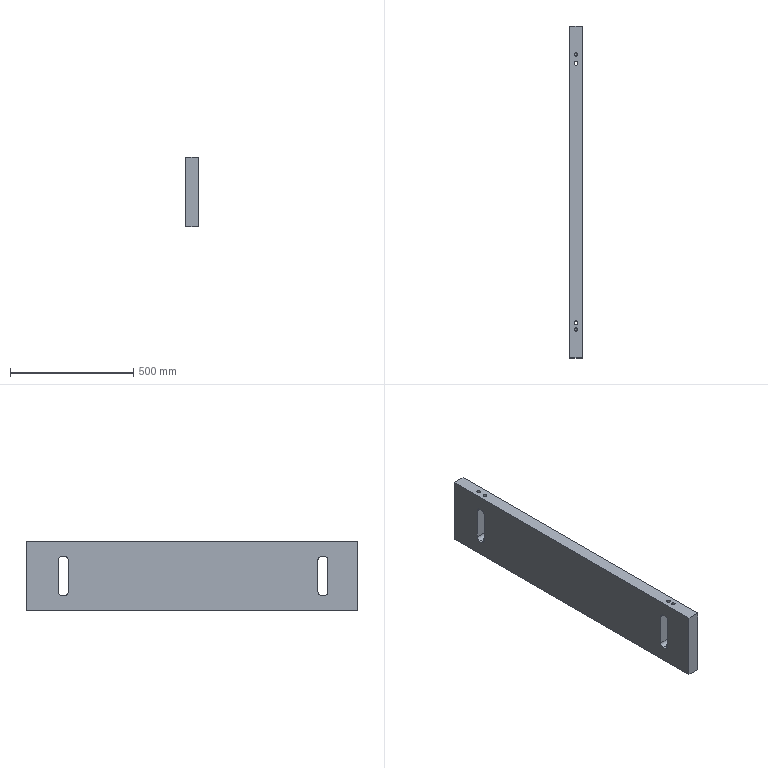Part | NX | features 29 2 | 1 solid | 38 faces | box 50 x 1345 x 280.5 mm | volume 18169896 mm3 | plane 18 | cylinder 16 | cone 4 | commonest cylinder face diameters 30 x8 14.1 x4 16.001 x4
STEP:
#1=CARTESIAN_POINT('',(3953.754,516.5,-273.));
#2=VERTEX_POINT('',#1);
#3=CARTESIAN_POINT('',(3966.246,516.5,-273.));
#4=VERTEX_POINT('',#3);
#5=CARTESIAN_POINT('',(3953.754,516.5,-273.));
#6=CARTESIAN_POINT('',(3955.263,514.616,-273.));
#7=CARTESIAN_POINT('',(3959.987,512.383,-273.606));
#8=CARTESIAN_POINT('',(3964.737,514.616,-273.));
#9=CARTESIAN_POINT('',(3966.246,516.5,-273.));
#10=B_SPLINE_CURVE_WITH_KNOTS('',3,(#5,#6,#7,#8,#9),.UNSPECIFIED.,.F.,.F.,(4,1,4),(0.,0.007135,0.01427),.UNSPECIFIED.);
#11=EDGE_CURVE('',#2,#4,#10,.T.);
#12=ORIENTED_EDGE('',*,*,#11,.F.);
#13=CARTESIAN_POINT('',(3953.754,526.5,-273.));
#14=VERTEX_POINT('',#13);
#15=CARTESIAN_POINT('',(3960.,521.5,-273.));
#16=DIRECTION('',(0.,0.,1.));
#17=DIRECTION('',(1.,0.,0.));
#18=AXIS2_PLACEMENT_3D('',#15,#16,#17);
#19=CIRCLE('',#18,8.001);
#20=EDGE_CURVE('',#14,#2,#19,.T.);
#21=ORIENTED_EDGE('',*,*,#20,.F.);
#22=CARTESIAN_POINT('',(3966.246,526.5,-273.));
#23=VERTEX_POINT('',#22);
#24=CARTESIAN_POINT('',(3966.246,526.5,-273.));
#25=CARTESIAN_POINT('',(3964.737,528.384,-273.));
#26=CARTESIAN_POINT('',(3960.013,530.617,-273.606));
#27=CARTESIAN_POINT('',(3955.263,528.384,-273.));
#28=CARTESIAN_POINT('',(3953.754,526.5,-273.));
#29=B_SPLINE_CURVE_WITH_KNOTS('',3,(#24,#25,#26,#27,#28),.UNSPECIFIED.,.F.,.F.,(4,1,4),(0.,0.007135,0.01427),.UNSPECIFIED.);
#30=EDGE_CURVE('',#23,#14,#29,.T.);
#31=ORIENTED_EDGE('',*,*,#30,.F.);
#32=CARTESIAN_POINT('',(3960.,521.5,-273.));
#33=DIRECTION('',(0.,0.,1.));
#34=DIRECTION('',(1.,0.,0.));
#35=AXIS2_PLACEMENT_3D('',#32,#33,#34);
#36=CIRCLE('',#35,8.001);
#37=EDGE_CURVE('',#4,#23,#36,.T.);
#38=ORIENTED_EDGE('',*,*,#37,.F.);
#39=EDGE_LOOP('',(#12,#21,#31,#38));
#40=FACE_BOUND('',#39,.T.);
#41=CARTESIAN_POINT('',(3968.001,521.5,-213.));
#42=VERTEX_POINT('',#41);
#43=CARTESIAN_POINT('',(3960.,521.5,-213.));
#44=DIRECTION('',(0.,0.,1.));
#45=DIRECTION('',(1.,0.,0.));
#46=AXIS2_PLACEMENT_3D('',#43,#44,#45);
#47=CIRCLE('',#46,8.001);
#48=EDGE_CURVE('',#42,#42,#47,.T.);
#49=ORIENTED_EDGE('',*,*,#48,.T.);
#50=EDGE_LOOP('',(#49));
#51=FACE_BOUND('',#50,.T.);
#52=CARTESIAN_POINT('',(3960.,521.5,-213.));
#53=DIRECTION('',(0.,0.,-1.));
#54=DIRECTION('',(-1.,0.,0.));
#55=AXIS2_PLACEMENT_3D('',#52,#53,#54);
#56=CYLINDRICAL_SURFACE('',#55,8.001);
#57=ADVANCED_FACE('',(#40,#51),#56,.F.);
#58=CARTESIAN_POINT('',(3960.,-557.5,-449.5));
#59=VERTEX_POINT('',#58);
#60=VERTEX_LOOP('',#59);
#61=FACE_BOUND('',#60,.T.);
#62=CARTESIAN_POINT('',(3967.05,-557.5,-456.55));
#63=VERTEX_POINT('',#62);
#64=CARTESIAN_POINT('',(3960.,-557.5,-456.55));
#65=DIRECTION('',(0.,0.,1.));
#66=DIRECTION('',(1.,0.,0.));
#67=AXIS2_PLACEMENT_3D('',#64,#65,#66);
#68=CIRCLE('',#67,7.05);
#69=EDGE_CURVE('',#63,#63,#68,.T.);
#70=ORIENTED_EDGE('',*,*,#69,.F.);
#71=EDGE_LOOP('',(#70));
#72=FACE_BOUND('',#71,.T.);
#73=CARTESIAN_POINT('',(3960.,-557.5,-456.55));
#74=DIRECTION('',(0.,0.,-1.));
#75=DIRECTION('',(1.,0.,0.));
#76=AXIS2_PLACEMENT_3D('',#73,#74,#75);
#77=CONICAL_SURFACE('',#76,7.05,0.7854);
#78=ADVANCED_FACE('',(#61,#72),#77,.F.);
#79=CARTESIAN_POINT('',(3960.,557.5,-449.5));
#80=VERTEX_POINT('',#79);
#81=VERTEX_LOOP('',#80);
#82=FACE_BOUND('',#81,.T.);
#83=CARTESIAN_POINT('',(3967.05,557.5,-456.55));
#84=VERTEX_POINT('',#83);
#85=CARTESIAN_POINT('',(3960.,557.5,-456.55));
#86=DIRECTION('',(0.,0.,1.));
#87=DIRECTION('',(1.,0.,0.));
#88=AXIS2_PLACEMENT_3D('',#85,#86,#87);
#89=CIRCLE('',#88,7.05);
#90=EDGE_CURVE('',#84,#84,#89,.T.);
#91=ORIENTED_EDGE('',*,*,#90,.F.);
#92=EDGE_LOOP('',(#91));
#93=FACE_BOUND('',#92,.T.);
#94=CARTESIAN_POINT('',(3960.,557.5,-456.55));
#95=DIRECTION('',(0.,0.,-1.));
#96=DIRECTION('',(1.,0.,0.));
#97=AXIS2_PLACEMENT_3D('',#94,#95,#96);
#98=CONICAL_SURFACE('',#97,7.05,0.7854);
#99=ADVANCED_FACE('',(#82,#93),#98,.F.);
#100=ORIENTED_EDGE('',*,*,#69,.T.);
#101=EDGE_LOOP('',(#100));
#102=FACE_BOUND('',#101,.T.);
#103=CARTESIAN_POINT('',(3967.05,-557.5,-493.5));
#104=VERTEX_POINT('',#103);
#105=CARTESIAN_POINT('',(3960.,-557.5,-493.5));
#106=DIRECTION('',(0.,0.,1.));
#107=DIRECTION('',(1.,0.,0.));
#108=AXIS2_PLACEMENT_3D('',#105,#106,#107);
#109=CIRCLE('',#108,7.05);
#110=EDGE_CURVE('',#104,#104,#109,.T.);
#111=ORIENTED_EDGE('',*,*,#110,.F.);
#112=EDGE_LOOP('',(#111));
#113=FACE_BOUND('',#112,.T.);
#114=CARTESIAN_POINT('',(3960.,-557.5,-493.5));
#115=DIRECTION('',(0.,0.,1.));
#116=DIRECTION('',(-1.,0.,0.));
#117=AXIS2_PLACEMENT_3D('',#114,#115,#116);
#118=CYLINDRICAL_SURFACE('',#117,7.05);
#119=ADVANCED_FACE('',(#102,#113),#118,.F.);
#120=ORIENTED_EDGE('',*,*,#90,.T.);
#121=EDGE_LOOP('',(#120));
#122=FACE_BOUND('',#121,.T.);
#123=CARTESIAN_POINT('',(3967.05,557.5,-493.5));
#124=VERTEX_POINT('',#123);
#125=CARTESIAN_POINT('',(3960.,557.5,-493.5));
#126=DIRECTION('',(0.,0.,1.));
#127=DIRECTION('',(1.,0.,0.));
#128=AXIS2_PLACEMENT_3D('',#125,#126,#127);
#129=CIRCLE('',#128,7.05);
#130=EDGE_CURVE('',#124,#124,#129,.T.);
#131=ORIENTED_EDGE('',*,*,#130,.F.);
#132=EDGE_LOOP('',(#131));
#133=FACE_BOUND('',#132,.T.);
#134=CARTESIAN_POINT('',(3960.,557.5,-493.5));
#135=DIRECTION('',(0.,0.,1.));
#136=DIRECTION('',(-1.,0.,0.));
#137=AXIS2_PLACEMENT_3D('',#134,#135,#136);
#138=CYLINDRICAL_SURFACE('',#137,7.05);
#139=ADVANCED_FACE('',(#122,#133),#138,.F.);
#140=CARTESIAN_POINT('',(3968.001,-530.5,-493.5));
#141=VERTEX_POINT('',#140);
#142=CARTESIAN_POINT('',(3960.,-530.5,-493.5));
#143=DIRECTION('',(0.,0.,1.));
#144=DIRECTION('',(1.,0.,0.));
#145=AXIS2_PLACEMENT_3D('',#142,#143,#144);
#146=CIRCLE('',#145,8.001);
#147=EDGE_CURVE('',#141,#141,#146,.T.);
#148=ORIENTED_EDGE('',*,*,#147,.F.);
#149=EDGE_LOOP('',(#148));
#150=FACE_BOUND('',#149,.T.);
#151=CARTESIAN_POINT('',(3953.754,-535.5,-433.));
#152=VERTEX_POINT('',#151);
#153=CARTESIAN_POINT('',(3953.754,-525.5,-433.));
#154=VERTEX_POINT('',#153);
#155=CARTESIAN_POINT('',(3960.,-530.5,-433.));
#156=DIRECTION('',(0.,0.,-1.));
#157=DIRECTION('',(-1.,0.,0.));
#158=AXIS2_PLACEMENT_3D('',#155,#156,#157);
#159=CIRCLE('',#158,8.001);
#160=EDGE_CURVE('',#152,#154,#159,.T.);
#161=ORIENTED_EDGE('',*,*,#160,.F.);
#162=CARTESIAN_POINT('',(3966.246,-535.5,-433.));
#163=VERTEX_POINT('',#162);
#164=CARTESIAN_POINT('',(3966.246,-535.5,-433.));
#165=CARTESIAN_POINT('',(3964.737,-537.384,-433.));
#166=CARTESIAN_POINT('',(3960.013,-539.617,-432.394));
#167=CARTESIAN_POINT('',(3955.263,-537.384,-433.));
#168=CARTESIAN_POINT('',(3953.754,-535.5,-433.));
#169=B_SPLINE_CURVE_WITH_KNOTS('',3,(#164,#165,#166,#167,#168),.UNSPECIFIED.,.F.,.F.,(4,1,4),(0.,0.007135,0.01427),.UNSPECIFIED.);
#170=EDGE_CURVE('',#163,#152,#169,.T.);
#171=ORIENTED_EDGE('',*,*,#170,.F.);
#172=CARTESIAN_POINT('',(3966.246,-525.5,-433.));
#173=VERTEX_POINT('',#172);
#174=CARTESIAN_POINT('',(3960.,-530.5,-433.));
#175=DIRECTION('',(0.,0.,-1.));
#176=DIRECTION('',(-1.,0.,0.));
#177=AXIS2_PLACEMENT_3D('',#174,#175,#176);
#178=CIRCLE('',#177,8.001);
#179=EDGE_CURVE('',#173,#163,#178,.T.);
#180=ORIENTED_EDGE('',*,*,#179,.F.);
#181=CARTESIAN_POINT('',(3953.754,-525.5,-433.));
#182=CARTESIAN_POINT('',(3955.263,-523.616,-433.));
#183=CARTESIAN_POINT('',(3959.987,-521.383,-432.394));
#184=CARTESIAN_POINT('',(3964.737,-523.616,-433.));
#185=CARTESIAN_POINT('',(3966.246,-525.5,-433.));
#186=B_SPLINE_CURVE_WITH_KNOTS('',3,(#181,#182,#183,#184,#185),.UNSPECIFIED.,.F.,.F.,(4,1,4),(0.,0.007135,0.01427),.UNSPECIFIED.);
#187=EDGE_CURVE('',#154,#173,#186,.T.);
#188=ORIENTED_EDGE('',*,*,#187,.F.);
#189=EDGE_LOOP('',(#161,#171,#180,#188));
#190=FACE_BOUND('',#189,.T.);
#191=CARTESIAN_POINT('',(3960.,-530.5,-493.5));
#192=DIRECTION('',(0.,0.,1.));
#193=DIRECTION('',(-1.,0.,0.));
#194=AXIS2_PLACEMENT_3D('',#191,#192,#193);
#195=CYLINDRICAL_SURFACE('',#194,8.001);
#196=ADVANCED_FACE('',(#150,#190),#195,.F.);
#197=CARTESIAN_POINT('',(3968.001,521.5,-493.5));
#198=VERTEX_POINT('',#197);
#199=CARTESIAN_POINT('',(3960.,521.5,-493.5));
#200=DIRECTION('',(0.,0.,1.));
#201=DIRECTION('',(1.,0.,0.));
#202=AXIS2_PLACEMENT_3D('',#199,#200,#201);
#203=CIRCLE('',#202,8.001);
#204=EDGE_CURVE('',#198,#198,#203,.T.);
#205=ORIENTED_EDGE('',*,*,#204,.F.);
#206=EDGE_LOOP('',(#205));
#207=FACE_BOUND('',#206,.T.);
#208=CARTESIAN_POINT('',(3953.754,516.5,-433.));
#209=VERTEX_POINT('',#208);
#210=CARTESIAN_POINT('',(3953.754,526.5,-433.));
#211=VERTEX_POINT('',#210);
#212=CARTESIAN_POINT('',(3960.,521.5,-433.));
#213=DIRECTION('',(0.,0.,-1.));
#214=DIRECTION('',(-1.,0.,0.));
#215=AXIS2_PLACEMENT_3D('',#212,#213,#214);
#216=CIRCLE('',#215,8.001);
#217=EDGE_CURVE('',#209,#211,#216,.T.);
#218=ORIENTED_EDGE('',*,*,#217,.F.);
#219=CARTESIAN_POINT('',(3966.246,516.5,-433.));
#220=VERTEX_POINT('',#219);
#221=CARTESIAN_POINT('',(3966.246,516.5,-433.));
#222=CARTESIAN_POINT('',(3964.737,514.616,-433.));
#223=CARTESIAN_POINT('',(3960.013,512.383,-432.394));
#224=CARTESIAN_POINT('',(3955.263,514.616,-433.));
#225=CARTESIAN_POINT('',(3953.754,516.5,-433.));
#226=B_SPLINE_CURVE_WITH_KNOTS('',3,(#221,#222,#223,#224,#225),.UNSPECIFIED.,.F.,.F.,(4,1,4),(0.,0.007135,0.01427),.UNSPECIFIED.);
#227=EDGE_CURVE('',#220,#209,#226,.T.);
#228=ORIENTED_EDGE('',*,*,#227,.F.);
#229=CARTESIAN_POINT('',(3966.246,526.5,-433.));
#230=VERTEX_POINT('',#229);
#231=CARTESIAN_POINT('',(3960.,521.5,-433.));
#232=DIRECTION('',(0.,0.,-1.));
#233=DIRECTION('',(-1.,0.,0.));
#234=AXIS2_PLACEMENT_3D('',#231,#232,#233);
#235=CIRCLE('',#234,8.001);
#236=EDGE_CURVE('',#230,#220,#235,.T.);
#237=ORIENTED_EDGE('',*,*,#236,.F.);
#238=CARTESIAN_POINT('',(3953.754,526.5,-433.));
#239=CARTESIAN_POINT('',(3955.263,528.384,-433.));
#240=CARTESIAN_POINT('',(3959.987,530.617,-432.394));
#241=CARTESIAN_POINT('',(3964.737,528.384,-433.));
#242=CARTESIAN_POINT('',(3966.246,526.5,-433.));
#243=B_SPLINE_CURVE_WITH_KNOTS('',3,(#238,#239,#240,#241,#242),.UNSPECIFIED.,.F.,.F.,(4,1,4),(0.,0.007135,0.01427),.UNSPECIFIED.);
#244=EDGE_CURVE('',#211,#230,#243,.T.);
#245=ORIENTED_EDGE('',*,*,#244,.F.);
#246=EDGE_LOOP('',(#218,#228,#237,#245));
#247=FACE_BOUND('',#246,.T.);
#248=CARTESIAN_POINT('',(3960.,521.5,-493.5));
#249=DIRECTION('',(0.,0.,1.));
#250=DIRECTION('',(-1.,0.,0.));
#251=AXIS2_PLACEMENT_3D('',#248,#249,#250);
#252=CYLINDRICAL_SURFACE('',#251,8.001);
#253=ADVANCED_FACE('',(#207,#247),#252,.F.);
#254=CARTESIAN_POINT('',(3960.,-557.5,-257.));
#255=VERTEX_POINT('',#254);
#256=VERTEX_LOOP('',#255);
#257=FACE_BOUND('',#256,.T.);
#258=CARTESIAN_POINT('',(3952.95,-557.5,-249.95));
#259=VERTEX_POINT('',#258);
#260=CARTESIAN_POINT('',(3960.,-557.5,-249.95));
#261=DIRECTION('',(0.,0.,-1.));
#262=DIRECTION('',(-1.,0.,0.));
#263=AXIS2_PLACEMENT_3D('',#260,#261,#262);
#264=CIRCLE('',#263,7.05);
#265=EDGE_CURVE('',#259,#259,#264,.T.);
#266=ORIENTED_EDGE('',*,*,#265,.F.);
#267=EDGE_LOOP('',(#266));
#268=FACE_BOUND('',#267,.T.);
#269=CARTESIAN_POINT('',(3960.,-557.5,-249.95));
#270=DIRECTION('',(0.,0.,1.));
#271=DIRECTION('',(-1.,0.,0.));
#272=AXIS2_PLACEMENT_3D('',#269,#270,#271);
#273=CONICAL_SURFACE('',#272,7.05,0.7854);
#274=ADVANCED_FACE('',(#257,#268),#273,.F.);
#275=CARTESIAN_POINT('',(3960.,557.5,-257.));
#276=VERTEX_POINT('',#275);
#277=VERTEX_LOOP('',#276);
#278=FACE_BOUND('',#277,.T.);
#279=CARTESIAN_POINT('',(3952.95,557.5,-249.95));
#280=VERTEX_POINT('',#279);
#281=CARTESIAN_POINT('',(3960.,557.5,-249.95));
#282=DIRECTION('',(0.,0.,-1.));
#283=DIRECTION('',(-1.,0.,0.));
#284=AXIS2_PLACEMENT_3D('',#281,#282,#283);
#285=CIRCLE('',#284,7.05);
#286=EDGE_CURVE('',#280,#280,#285,.T.);
#287=ORIENTED_EDGE('',*,*,#286,.F.);
#288=EDGE_LOOP('',(#287));
#289=FACE_BOUND('',#288,.T.);
#290=CARTESIAN_POINT('',(3960.,557.5,-249.95));
#291=DIRECTION('',(0.,0.,1.));
#292=DIRECTION('',(-1.,0.,0.));
#293=AXIS2_PLACEMENT_3D('',#290,#291,#292);
#294=CONICAL_SURFACE('',#293,7.05,0.7854);
#295=ADVANCED_FACE('',(#278,#289),#294,.F.);
#296=CARTESIAN_POINT('',(3985.,-525.5,-433.));
#297=VERTEX_POINT('',#296);
#298=CARTESIAN_POINT('',(3960.,-525.5,-433.));
#299=DIRECTION('',(1.,0.,0.));
#300=VECTOR('',#299,1000.);
#301=LINE('',#298,#300);
#302=EDGE_CURVE('',#173,#297,#301,.T.);
#303=ORIENTED_EDGE('',*,*,#302,.F.);
#304=ORIENTED_EDGE('',*,*,#179,.T.);
#305=CARTESIAN_POINT('',(3985.,-535.5,-433.));
#306=VERTEX_POINT('',#305);
#307=CARTESIAN_POINT('',(3960.,-535.5,-433.));
#308=DIRECTION('',(-1.,0.,0.));
#309=VECTOR('',#308,1000.);
#310=LINE('',#307,#309);
#311=EDGE_CURVE('',#306,#163,#310,.T.);
#312=ORIENTED_EDGE('',*,*,#311,.F.);
#313=CARTESIAN_POINT('',(3985.,193.,-433.));
#314=DIRECTION('',(0.,1.,0.));
#315=VECTOR('',#314,1000.);
#316=LINE('',#313,#315);
#317=EDGE_CURVE('',#306,#297,#316,.T.);
#318=ORIENTED_EDGE('',*,*,#317,.T.);
#319=EDGE_LOOP('',(#303,#304,#312,#318));
#320=FACE_BOUND('',#319,.T.);
#321=CARTESIAN_POINT('',(3960.,-521.5,-433.));
#322=DIRECTION('',(0.,0.,-1.));
#323=DIRECTION('',(-1.,0.,0.));
#324=AXIS2_PLACEMENT_3D('',#321,#322,#323);
#325=PLANE('',#324);
#326=ADVANCED_FACE('',(#320),#325,.F.);
#327=CARTESIAN_POINT('',(3985.,526.5,-433.));
#328=VERTEX_POINT('',#327);
#329=CARTESIAN_POINT('',(3960.,526.5,-433.));
#330=DIRECTION('',(-1.,0.,0.));
#331=VECTOR('',#330,1000.);
#332=LINE('',#329,#331);
#333=EDGE_CURVE('',#328,#230,#332,.T.);
#334=ORIENTED_EDGE('',*,*,#333,.T.);
#335=ORIENTED_EDGE('',*,*,#236,.T.);
#336=CARTESIAN_POINT('',(3985.,516.5,-433.));
#337=VERTEX_POINT('',#336);
#338=CARTESIAN_POINT('',(3960.,516.5,-433.));
#339=DIRECTION('',(1.,0.,0.));
#340=VECTOR('',#339,1000.);
#341=LINE('',#338,#340);
#342=EDGE_CURVE('',#220,#337,#341,.T.);
#343=ORIENTED_EDGE('',*,*,#342,.T.);
#344=CARTESIAN_POINT('',(3985.,193.,-433.));
#345=DIRECTION('',(0.,1.,0.));
#346=VECTOR('',#345,1000.);
#347=LINE('',#344,#346);
#348=EDGE_CURVE('',#337,#328,#347,.T.);
#349=ORIENTED_EDGE('',*,*,#348,.T.);
#350=EDGE_LOOP('',(#334,#335,#343,#349));
#351=FACE_BOUND('',#350,.T.);
#352=CARTESIAN_POINT('',(3960.,521.5,-433.));
#353=DIRECTION('',(0.,0.,-1.));
#354=DIRECTION('',(-1.,0.,0.));
#355=AXIS2_PLACEMENT_3D('',#352,#353,#354);
#356=PLANE('',#355);
#357=ADVANCED_FACE('',(#351),#356,.F.);
#358=ORIENTED_EDGE('',*,*,#147,.T.);
#359=EDGE_LOOP('',(#358));
#360=FACE_BOUND('',#359,.T.);
#361=ORIENTED_EDGE('',*,*,#130,.T.);
#362=EDGE_LOOP('',(#361));
#363=FACE_BOUND('',#362,.T.);
#364=CARTESIAN_POINT('',(3935.,672.5,-493.5));
#365=VERTEX_POINT('',#364);
#366=CARTESIAN_POINT('',(3935.,-672.5,-493.5));
#367=VERTEX_POINT('',#366);
#368=CARTESIAN_POINT('',(3935.,193.,-493.5));
#369=DIRECTION('',(0.,-1.,0.));
#370=VECTOR('',#369,1000.);
#371=LINE('',#368,#370);
#372=EDGE_CURVE('',#365,#367,#371,.T.);
#373=ORIENTED_EDGE('',*,*,#372,.F.);
#374=CARTESIAN_POINT('',(3985.,672.5,-493.5));
#375=VERTEX_POINT('',#374);
#376=CARTESIAN_POINT('',(1822.5,672.5,-493.5));
#377=DIRECTION('',(1.,0.,0.));
#378=VECTOR('',#377,1000.);
#379=LINE('',#376,#378);
#380=EDGE_CURVE('',#365,#375,#379,.T.);
#381=ORIENTED_EDGE('',*,*,#380,.T.);
#382=CARTESIAN_POINT('',(3985.,-672.5,-493.5));
#383=VERTEX_POINT('',#382);
#384=CARTESIAN_POINT('',(3985.,193.,-493.5));
#385=DIRECTION('',(0.,1.,0.));
#386=VECTOR('',#385,1000.);
#387=LINE('',#384,#386);
#388=EDGE_CURVE('',#383,#375,#387,.T.);
#389=ORIENTED_EDGE('',*,*,#388,.F.);
#390=CARTESIAN_POINT('',(4325.,-672.5,-493.5));
#391=DIRECTION('',(-1.,0.,0.));
#392=VECTOR('',#391,1000.);
#393=LINE('',#390,#392);
#394=EDGE_CURVE('',#383,#367,#393,.T.);
#395=ORIENTED_EDGE('',*,*,#394,.T.);
#396=EDGE_LOOP('',(#373,#381,#389,#395));
#397=FACE_BOUND('',#396,.T.);
#398=ORIENTED_EDGE('',*,*,#110,.T.);
#399=EDGE_LOOP('',(#398));
#400=FACE_BOUND('',#399,.T.);
#401=ORIENTED_EDGE('',*,*,#204,.T.);
#402=EDGE_LOOP('',(#401));
#403=FACE_BOUND('',#402,.T.);
#404=CARTESIAN_POINT('',(1945.,0.,-493.5));
#405=DIRECTION('',(0.,0.,-1.));
#406=DIRECTION('',(1.,0.,0.));
#407=AXIS2_PLACEMENT_3D('',#404,#405,#406);
#408=PLANE('',#407);
#409=ADVANCED_FACE('',(#360,#363,#397,#400,#403),#408,.T.);
#410=CARTESIAN_POINT('',(3935.,-525.5,-433.));
#411=VERTEX_POINT('',#410);
#412=CARTESIAN_POINT('',(3960.,-525.5,-433.));
#413=DIRECTION('',(1.,0.,0.));
#414=VECTOR('',#413,1000.);
#415=LINE('',#412,#414);
#416=EDGE_CURVE('',#411,#154,#415,.T.);
#417=ORIENTED_EDGE('',*,*,#416,.T.);
#418=ORIENTED_EDGE('',*,*,#187,.T.);
#419=ORIENTED_EDGE('',*,*,#302,.T.);
#420=CARTESIAN_POINT('',(3985.,-510.5,-418.));
#421=VERTEX_POINT('',#420);
#422=CARTESIAN_POINT('',(3985.,-525.5,-418.));
#423=DIRECTION('',(1.,0.,0.));
#424=DIRECTION('',(0.,0.,-1.));
#425=AXIS2_PLACEMENT_3D('',#422,#423,#424);
#426=CIRCLE('',#425,15.);
#427=EDGE_CURVE('',#297,#421,#426,.T.);
#428=ORIENTED_EDGE('',*,*,#427,.T.);
#429=CARTESIAN_POINT('',(3935.,-510.5,-418.));
#430=VERTEX_POINT('',#429);
#431=CARTESIAN_POINT('',(3960.,-510.5,-418.));
#432=DIRECTION('',(-1.,0.,0.));
#433=VECTOR('',#432,1000.);
#434=LINE('',#431,#433);
#435=EDGE_CURVE('',#421,#430,#434,.T.);
#436=ORIENTED_EDGE('',*,*,#435,.T.);
#437=CARTESIAN_POINT('',(3935.,-525.5,-418.));
#438=DIRECTION('',(-1.,0.,0.));
#439=DIRECTION('',(0.,0.,1.));
#440=AXIS2_PLACEMENT_3D('',#437,#438,#439);
#441=CIRCLE('',#440,15.);
#442=EDGE_CURVE('',#430,#411,#441,.T.);
#443=ORIENTED_EDGE('',*,*,#442,.T.);
#444=EDGE_LOOP('',(#417,#418,#419,#428,#436,#443));
#445=FACE_BOUND('',#444,.T.);
#446=CARTESIAN_POINT('',(3960.,-525.5,-418.));
#447=DIRECTION('',(1.,0.,0.));
#448=DIRECTION('',(0.,0.,-1.));
#449=AXIS2_PLACEMENT_3D('',#446,#447,#448);
#450=CYLINDRICAL_SURFACE('',#449,15.);
#451=ADVANCED_FACE('',(#445),#450,.F.);
#452=CARTESIAN_POINT('',(3935.,-535.5,-433.));
#453=VERTEX_POINT('',#452);
#454=CARTESIAN_POINT('',(3960.,-535.5,-433.));
#455=DIRECTION('',(-1.,0.,0.));
#456=VECTOR('',#455,1000.);
#457=LINE('',#454,#456);
#458=EDGE_CURVE('',#152,#453,#457,.T.);
#459=ORIENTED_EDGE('',*,*,#458,.F.);
#460=ORIENTED_EDGE('',*,*,#160,.T.);
#461=ORIENTED_EDGE('',*,*,#416,.F.);
#462=CARTESIAN_POINT('',(3935.,193.,-433.));
#463=DIRECTION('',(0.,-1.,0.));
#464=VECTOR('',#463,1000.);
#465=LINE('',#462,#464);
#466=EDGE_CURVE('',#411,#453,#465,.T.);
#467=ORIENTED_EDGE('',*,*,#466,.T.);
#468=EDGE_LOOP('',(#459,#460,#461,#467));
#469=FACE_BOUND('',#468,.T.);
#470=CARTESIAN_POINT('',(3960.,-521.5,-433.));
#471=DIRECTION('',(0.,0.,-1.));
#472=DIRECTION('',(-1.,0.,0.));
#473=AXIS2_PLACEMENT_3D('',#470,#471,#472);
#474=PLANE('',#473);
#475=ADVANCED_FACE('',(#469),#474,.F.);
#476=ORIENTED_EDGE('',*,*,#311,.T.);
#477=ORIENTED_EDGE('',*,*,#170,.T.);
#478=ORIENTED_EDGE('',*,*,#458,.T.);
#479=CARTESIAN_POINT('',(3935.,-550.5,-418.));
#480=VERTEX_POINT('',#479);
#481=CARTESIAN_POINT('',(3935.,-535.5,-418.));
#482=DIRECTION('',(-1.,0.,0.));
#483=DIRECTION('',(0.,0.,1.));
#484=AXIS2_PLACEMENT_3D('',#481,#482,#483);
#485=CIRCLE('',#484,15.);
#486=EDGE_CURVE('',#453,#480,#485,.T.);
#487=ORIENTED_EDGE('',*,*,#486,.T.);
#488=CARTESIAN_POINT('',(3985.,-550.5,-418.));
#489=VERTEX_POINT('',#488);
#490=CARTESIAN_POINT('',(3960.,-550.5,-418.));
#491=DIRECTION('',(1.,0.,0.));
#492=VECTOR('',#491,1000.);
#493=LINE('',#490,#492);
#494=EDGE_CURVE('',#480,#489,#493,.T.);
#495=ORIENTED_EDGE('',*,*,#494,.T.);
#496=CARTESIAN_POINT('',(3985.,-535.5,-418.));
#497=DIRECTION('',(1.,0.,0.));
#498=DIRECTION('',(0.,0.,-1.));
#499=AXIS2_PLACEMENT_3D('',#496,#497,#498);
#500=CIRCLE('',#499,15.);
#501=EDGE_CURVE('',#489,#306,#500,.T.);
#502=ORIENTED_EDGE('',*,*,#501,.T.);
#503=EDGE_LOOP('',(#476,#477,#478,#487,#495,#502));
#504=FACE_BOUND('',#503,.T.);
#505=CARTESIAN_POINT('',(3960.,-535.5,-418.));
#506=DIRECTION('',(-1.,0.,0.));
#507=DIRECTION('',(0.,0.,1.));
#508=AXIS2_PLACEMENT_3D('',#505,#506,#507);
#509=CYLINDRICAL_SURFACE('',#508,15.);
#510=ADVANCED_FACE('',(#504),#509,.F.);
#511=CARTESIAN_POINT('',(3935.,526.5,-433.));
#512=VERTEX_POINT('',#511);
#513=CARTESIAN_POINT('',(3960.,526.5,-433.));
#514=DIRECTION('',(-1.,0.,0.));
#515=VECTOR('',#514,1000.);
#516=LINE('',#513,#515);
#517=EDGE_CURVE('',#211,#512,#516,.T.);
#518=ORIENTED_EDGE('',*,*,#517,.F.);
#519=ORIENTED_EDGE('',*,*,#244,.T.);
#520=ORIENTED_EDGE('',*,*,#333,.F.);
#521=CARTESIAN_POINT('',(3985.,541.5,-418.));
#522=VERTEX_POINT('',#521);
#523=CARTESIAN_POINT('',(3985.,526.5,-418.));
#524=DIRECTION('',(1.,0.,0.));
#525=DIRECTION('',(0.,0.,-1.));
#526=AXIS2_PLACEMENT_3D('',#523,#524,#525);
#527=CIRCLE('',#526,15.);
#528=EDGE_CURVE('',#328,#522,#527,.T.);
#529=ORIENTED_EDGE('',*,*,#528,.T.);
#530=CARTESIAN_POINT('',(3935.,541.5,-418.));
#531=VERTEX_POINT('',#530);
#532=CARTESIAN_POINT('',(3960.,541.5,-418.));
#533=DIRECTION('',(1.,0.,0.));
#534=VECTOR('',#533,1000.);
#535=LINE('',#532,#534);
#536=EDGE_CURVE('',#531,#522,#535,.T.);
#537=ORIENTED_EDGE('',*,*,#536,.F.);
#538=CARTESIAN_POINT('',(3935.,526.5,-418.));
#539=DIRECTION('',(-1.,0.,0.));
#540=DIRECTION('',(0.,0.,1.));
#541=AXIS2_PLACEMENT_3D('',#538,#539,#540);
#542=CIRCLE('',#541,15.);
#543=EDGE_CURVE('',#531,#512,#542,.T.);
#544=ORIENTED_EDGE('',*,*,#543,.T.);
#545=EDGE_LOOP('',(#518,#519,#520,#529,#537,#544));
#546=FACE_BOUND('',#545,.T.);
#547=CARTESIAN_POINT('',(3960.,526.5,-418.));
#548=DIRECTION('',(-1.,0.,0.));
#549=DIRECTION('',(0.,0.,1.));
#550=AXIS2_PLACEMENT_3D('',#547,#548,#549);
#551=CYLINDRICAL_SURFACE('',#550,15.);
#552=ADVANCED_FACE('',(#546),#551,.F.);
#553=CARTESIAN_POINT('',(3935.,516.5,-433.));
#554=VERTEX_POINT('',#553);
#555=CARTESIAN_POINT('',(3960.,516.5,-433.));
#556=DIRECTION('',(1.,0.,0.));
#557=VECTOR('',#556,1000.);
#558=LINE('',#555,#557);
#559=EDGE_CURVE('',#554,#209,#558,.T.);
#560=ORIENTED_EDGE('',*,*,#559,.T.);
#561=ORIENTED_EDGE('',*,*,#217,.T.);
#562=ORIENTED_EDGE('',*,*,#517,.T.);
#563=CARTESIAN_POINT('',(3935.,193.,-433.));
#564=DIRECTION('',(0.,-1.,0.));
#565=VECTOR('',#564,1000.);
#566=LINE('',#563,#565);
#567=EDGE_CURVE('',#512,#554,#566,.T.);
#568=ORIENTED_EDGE('',*,*,#567,.T.);
#569=EDGE_LOOP('',(#560,#561,#562,#568));
#570=FACE_BOUND('',#569,.T.);
#571=CARTESIAN_POINT('',(3960.,521.5,-433.));
#572=DIRECTION('',(0.,0.,-1.));
#573=DIRECTION('',(-1.,0.,0.));
#574=AXIS2_PLACEMENT_3D('',#571,#572,#573);
#575=PLANE('',#574);
#576=ADVANCED_FACE('',(#570),#575,.F.);
#577=ORIENTED_EDGE('',*,*,#342,.F.);
#578=ORIENTED_EDGE('',*,*,#227,.T.);
#579=ORIENTED_EDGE('',*,*,#559,.F.);
#580=CARTESIAN_POINT('',(3935.,501.5,-418.));
#581=VERTEX_POINT('',#580);
#582=CARTESIAN_POINT('',(3935.,516.5,-418.));
#583=DIRECTION('',(-1.,0.,0.));
#584=DIRECTION('',(0.,0.,1.));
#585=AXIS2_PLACEMENT_3D('',#582,#583,#584);
#586=CIRCLE('',#585,15.);
#587=EDGE_CURVE('',#554,#581,#586,.T.);
#588=ORIENTED_EDGE('',*,*,#587,.T.);
#589=CARTESIAN_POINT('',(3985.,501.5,-418.));
#590=VERTEX_POINT('',#589);
#591=CARTESIAN_POINT('',(3960.,501.5,-418.));
#592=DIRECTION('',(-1.,0.,0.));
#593=VECTOR('',#592,1000.);
#594=LINE('',#591,#593);
#595=EDGE_CURVE('',#590,#581,#594,.T.);
#596=ORIENTED_EDGE('',*,*,#595,.F.);
#597=CARTESIAN_POINT('',(3985.,516.5,-418.));
#598=DIRECTION('',(1.,0.,0.));
#599=DIRECTION('',(0.,0.,-1.));
#600=AXIS2_PLACEMENT_3D('',#597,#598,#599);
#601=CIRCLE('',#600,15.);
#602=EDGE_CURVE('',#590,#337,#601,.T.);
#603=ORIENTED_EDGE('',*,*,#602,.T.);
#604=EDGE_LOOP('',(#577,#578,#579,#588,#596,#603));
#605=FACE_BOUND('',#604,.T.);
#606=CARTESIAN_POINT('',(3960.,516.5,-418.));
#607=DIRECTION('',(1.,0.,0.));
#608=DIRECTION('',(0.,0.,-1.));
#609=AXIS2_PLACEMENT_3D('',#606,#607,#608);
#610=CYLINDRICAL_SURFACE('',#609,15.);
#611=ADVANCED_FACE('',(#605),#610,.F.);
#612=ORIENTED_EDGE('',*,*,#265,.T.);
#613=EDGE_LOOP('',(#612));
#614=FACE_BOUND('',#613,.T.);
#615=CARTESIAN_POINT('',(3967.05,-557.5,-213.));
#616=VERTEX_POINT('',#615);
#617=CARTESIAN_POINT('',(3960.,-557.5,-213.));
#618=DIRECTION('',(0.,0.,-1.));
#619=DIRECTION('',(1.,0.,0.));
#620=AXIS2_PLACEMENT_3D('',#617,#618,#619);
#621=CIRCLE('',#620,7.05);
#622=EDGE_CURVE('',#616,#616,#621,.T.);
#623=ORIENTED_EDGE('',*,*,#622,.F.);
#624=EDGE_LOOP('',(#623));
#625=FACE_BOUND('',#624,.T.);
#626=CARTESIAN_POINT('',(3960.,-557.5,-213.));
#627=DIRECTION('',(0.,0.,-1.));
#628=DIRECTION('',(-1.,0.,0.));
#629=AXIS2_PLACEMENT_3D('',#626,#627,#628);
#630=CYLINDRICAL_SURFACE('',#629,7.05);
#631=ADVANCED_FACE('',(#614,#625),#630,.F.);
#632=ORIENTED_EDGE('',*,*,#380,.F.);
#633=CARTESIAN_POINT('',(3935.,672.5,-213.));
#634=VERTEX_POINT('',#633);
#635=CARTESIAN_POINT('',(3935.,672.5,-205.5));
#636=DIRECTION('',(0.,0.,1.));
#637=VECTOR('',#636,1000.);
#638=LINE('',#635,#637);
#639=EDGE_CURVE('',#365,#634,#638,.T.);
#640=ORIENTED_EDGE('',*,*,#639,.T.);
#641=CARTESIAN_POINT('',(3985.,672.5,-213.));
#642=VERTEX_POINT('',#641);
#643=CARTESIAN_POINT('',(1822.5,672.5,-213.));
#644=DIRECTION('',(-1.,0.,0.));
#645=VECTOR('',#644,1000.);
#646=LINE('',#643,#645);
#647=EDGE_CURVE('',#642,#634,#646,.T.);
#648=ORIENTED_EDGE('',*,*,#647,.F.);
#649=CARTESIAN_POINT('',(3985.,672.5,-205.5));
#650=DIRECTION('',(0.,0.,1.));
#651=VECTOR('',#650,1000.);
#652=LINE('',#649,#651);
#653=EDGE_CURVE('',#375,#642,#652,.T.);
#654=ORIENTED_EDGE('',*,*,#653,.F.);
#655=EDGE_LOOP('',(#632,#640,#648,#654));
#656=FACE_BOUND('',#655,.T.);
#657=CARTESIAN_POINT('',(1822.5,672.5,91.));
#658=DIRECTION('',(0.,-1.,0.));
#659=DIRECTION('',(-1.,0.,0.));
#660=AXIS2_PLACEMENT_3D('',#657,#658,#659);
#661=PLANE('',#660);
#662=ADVANCED_FACE('',(#656),#661,.F.);
#663=ORIENTED_EDGE('',*,*,#394,.F.);
#664=CARTESIAN_POINT('',(3985.,-672.5,-213.));
#665=VERTEX_POINT('',#664);
#666=CARTESIAN_POINT('',(3985.,-672.5,-543.5));
#667=DIRECTION('',(0.,0.,1.));
#668=VECTOR('',#667,1000.);
#669=LINE('',#666,#668);
#670=EDGE_CURVE('',#383,#665,#669,.T.);
#671=ORIENTED_EDGE('',*,*,#670,.T.);
#672=CARTESIAN_POINT('',(3935.,-672.5,-213.));
#673=VERTEX_POINT('',#672);
#674=CARTESIAN_POINT('',(4325.,-672.5,-213.));
#675=DIRECTION('',(1.,0.,0.));
#676=VECTOR('',#675,1000.);
#677=LINE('',#674,#676);
#678=EDGE_CURVE('',#673,#665,#677,.T.);
#679=ORIENTED_EDGE('',*,*,#678,.F.);
#680=CARTESIAN_POINT('',(3935.,-672.5,-113.));
#681=DIRECTION('',(0.,0.,1.));
#682=VECTOR('',#681,1000.);
#683=LINE('',#680,#682);
#684=EDGE_CURVE('',#367,#673,#683,.T.);
#685=ORIENTED_EDGE('',*,*,#684,.F.);
#686=EDGE_LOOP('',(#663,#671,#679,#685));
#687=FACE_BOUND('',#686,.T.);
#688=CARTESIAN_POINT('',(4325.,-672.5,-113.));
#689=DIRECTION('',(0.,1.,0.));
#690=DIRECTION('',(1.,0.,0.));
#691=AXIS2_PLACEMENT_3D('',#688,#689,#690);
#692=PLANE('',#691);
#693=ADVANCED_FACE('',(#687),#692,.F.);
#694=CARTESIAN_POINT('',(3935.,-510.5,-288.));
#695=VERTEX_POINT('',#694);
#696=CARTESIAN_POINT('',(3935.,-510.5,-205.5));
#697=DIRECTION('',(0.,0.,-1.));
#698=VECTOR('',#697,1000.);
#699=LINE('',#696,#698);
#700=EDGE_CURVE('',#695,#430,#699,.T.);
#701=ORIENTED_EDGE('',*,*,#700,.T.);
#702=ORIENTED_EDGE('',*,*,#435,.F.);
#703=CARTESIAN_POINT('',(3985.,-510.5,-288.));
#704=VERTEX_POINT('',#703);
#705=CARTESIAN_POINT('',(3985.,-510.5,-205.5));
#706=DIRECTION('',(0.,0.,1.));
#707=VECTOR('',#706,1000.);
#708=LINE('',#705,#707);
#709=EDGE_CURVE('',#421,#704,#708,.T.);
#710=ORIENTED_EDGE('',*,*,#709,.T.);
#711=CARTESIAN_POINT('',(3960.,-510.5,-288.));
#712=DIRECTION('',(1.,0.,0.));
#713=VECTOR('',#712,1000.);
#714=LINE('',#711,#713);
#715=EDGE_CURVE('',#695,#704,#714,.T.);
#716=ORIENTED_EDGE('',*,*,#715,.F.);
#717=EDGE_LOOP('',(#701,#702,#710,#716));
#718=FACE_BOUND('',#717,.T.);
#719=CARTESIAN_POINT('',(3960.,-510.5,-353.));
#720=DIRECTION('',(0.,1.,0.));
#721=DIRECTION('',(0.,0.,-1.));
#722=AXIS2_PLACEMENT_3D('',#719,#720,#721);
#723=PLANE('',#722);
#724=ADVANCED_FACE('',(#718),#723,.F.);
#725=CARTESIAN_POINT('',(3935.,-550.5,-288.));
#726=VERTEX_POINT('',#725);
#727=CARTESIAN_POINT('',(3935.,-550.5,-205.5));
#728=DIRECTION('',(0.,0.,1.));
#729=VECTOR('',#728,1000.);
#730=LINE('',#727,#729);
#731=EDGE_CURVE('',#480,#726,#730,.T.);
#732=ORIENTED_EDGE('',*,*,#731,.T.);
#733=CARTESIAN_POINT('',(3985.,-550.5,-288.));
#734=VERTEX_POINT('',#733);
#735=CARTESIAN_POINT('',(3960.,-550.5,-288.));
#736=DIRECTION('',(-1.,0.,0.));
#737=VECTOR('',#736,1000.);
#738=LINE('',#735,#737);
#739=EDGE_CURVE('',#734,#726,#738,.T.);
#740=ORIENTED_EDGE('',*,*,#739,.F.);
#741=CARTESIAN_POINT('',(3985.,-550.5,-205.5));
#742=DIRECTION('',(0.,0.,-1.));
#743=VECTOR('',#742,1000.);
#744=LINE('',#741,#743);
#745=EDGE_CURVE('',#734,#489,#744,.T.);
#746=ORIENTED_EDGE('',*,*,#745,.T.);
#747=ORIENTED_EDGE('',*,*,#494,.F.);
#748=EDGE_LOOP('',(#732,#740,#746,#747));
#749=FACE_BOUND('',#748,.T.);
#750=CARTESIAN_POINT('',(3960.,-550.5,-353.));
#751=DIRECTION('',(0.,-1.,0.));
#752=DIRECTION('',(0.,0.,1.));
#753=AXIS2_PLACEMENT_3D('',#750,#751,#752);
#754=PLANE('',#753);
#755=ADVANCED_FACE('',(#749),#754,.F.);
#756=CARTESIAN_POINT('',(3935.,501.5,-288.));
#757=VERTEX_POINT('',#756);
#758=CARTESIAN_POINT('',(3935.,501.5,-205.5));
#759=DIRECTION('',(0.,0.,1.));
#760=VECTOR('',#759,1000.);
#761=LINE('',#758,#760);
#762=EDGE_CURVE('',#581,#757,#761,.T.);
#763=ORIENTED_EDGE('',*,*,#762,.T.);
#764=CARTESIAN_POINT('',(3985.,501.5,-288.));
#765=VERTEX_POINT('',#764);
#766=CARTESIAN_POINT('',(3960.,501.5,-288.));
#767=DIRECTION('',(1.,0.,0.));
#768=VECTOR('',#767,1000.);
#769=LINE('',#766,#768);
#770=EDGE_CURVE('',#757,#765,#769,.T.);
#771=ORIENTED_EDGE('',*,*,#770,.T.);
#772=CARTESIAN_POINT('',(3985.,501.5,-205.5));
#773=DIRECTION('',(0.,0.,-1.));
#774=VECTOR('',#773,1000.);
#775=LINE('',#772,#774);
#776=EDGE_CURVE('',#765,#590,#775,.T.);
#777=ORIENTED_EDGE('',*,*,#776,.T.);
#778=ORIENTED_EDGE('',*,*,#595,.T.);
#779=EDGE_LOOP('',(#763,#771,#777,#778));
#780=FACE_BOUND('',#779,.T.);
#781=CARTESIAN_POINT('',(3960.,501.5,-353.));
#782=DIRECTION('',(0.,-1.,0.));
#783=DIRECTION('',(0.,0.,-1.));
#784=AXIS2_PLACEMENT_3D('',#781,#782,#783);
#785=PLANE('',#784);
#786=ADVANCED_FACE('',(#780),#785,.F.);
#787=CARTESIAN_POINT('',(3985.,516.5,-273.));
#788=VERTEX_POINT('',#787);
#789=CARTESIAN_POINT('',(3985.,516.5,-288.));
#790=DIRECTION('',(1.,0.,0.));
#791=DIRECTION('',(0.,0.,-1.));
#792=AXIS2_PLACEMENT_3D('',#789,#790,#791);
#793=CIRCLE('',#792,15.);
#794=EDGE_CURVE('',#788,#765,#793,.T.);
#795=ORIENTED_EDGE('',*,*,#794,.F.);
#796=CARTESIAN_POINT('',(3985.,526.5,-273.));
#797=VERTEX_POINT('',#796);
#798=CARTESIAN_POINT('',(3985.,193.,-273.));
#799=DIRECTION('',(0.,-1.,0.));
#800=VECTOR('',#799,1000.);
#801=LINE('',#798,#800);
#802=EDGE_CURVE('',#797,#788,#801,.T.);
#803=ORIENTED_EDGE('',*,*,#802,.F.);
#804=CARTESIAN_POINT('',(3985.,541.5,-288.));
#805=VERTEX_POINT('',#804);
#806=CARTESIAN_POINT('',(3985.,526.5,-288.));
#807=DIRECTION('',(1.,0.,0.));
#808=DIRECTION('',(0.,0.,-1.));
#809=AXIS2_PLACEMENT_3D('',#806,#807,#808);
#810=CIRCLE('',#809,15.);
#811=EDGE_CURVE('',#805,#797,#810,.T.);
#812=ORIENTED_EDGE('',*,*,#811,.F.);
#813=CARTESIAN_POINT('',(3985.,541.5,-205.5));
#814=DIRECTION('',(0.,0.,1.));
#815=VECTOR('',#814,1000.);
#816=LINE('',#813,#815);
#817=EDGE_CURVE('',#522,#805,#816,.T.);
#818=ORIENTED_EDGE('',*,*,#817,.F.);
#819=ORIENTED_EDGE('',*,*,#528,.F.);
#820=ORIENTED_EDGE('',*,*,#348,.F.);
#821=ORIENTED_EDGE('',*,*,#602,.F.);
#822=ORIENTED_EDGE('',*,*,#776,.F.);
#823=EDGE_LOOP('',(#795,#803,#812,#818,#819,#820,#821,#822));
#824=FACE_BOUND('',#823,.T.);
#825=CARTESIAN_POINT('',(3985.,-525.5,-273.));
#826=VERTEX_POINT('',#825);
#827=CARTESIAN_POINT('',(3985.,-525.5,-288.));
#828=DIRECTION('',(1.,0.,0.));
#829=DIRECTION('',(0.,0.,-1.));
#830=AXIS2_PLACEMENT_3D('',#827,#828,#829);
#831=CIRCLE('',#830,15.);
#832=EDGE_CURVE('',#704,#826,#831,.T.);
#833=ORIENTED_EDGE('',*,*,#832,.F.);
#834=ORIENTED_EDGE('',*,*,#709,.F.);
#835=ORIENTED_EDGE('',*,*,#427,.F.);
#836=ORIENTED_EDGE('',*,*,#317,.F.);
#837=ORIENTED_EDGE('',*,*,#501,.F.);
#838=ORIENTED_EDGE('',*,*,#745,.F.);
#839=CARTESIAN_POINT('',(3985.,-535.5,-273.));
#840=VERTEX_POINT('',#839);
#841=CARTESIAN_POINT('',(3985.,-535.5,-288.));
#842=DIRECTION('',(1.,0.,0.));
#843=DIRECTION('',(0.,0.,-1.));
#844=AXIS2_PLACEMENT_3D('',#841,#842,#843);
#845=CIRCLE('',#844,15.);
#846=EDGE_CURVE('',#840,#734,#845,.T.);
#847=ORIENTED_EDGE('',*,*,#846,.F.);
#848=CARTESIAN_POINT('',(3985.,193.,-273.));
#849=DIRECTION('',(0.,-1.,0.));
#850=VECTOR('',#849,1000.);
#851=LINE('',#848,#850);
#852=EDGE_CURVE('',#826,#840,#851,.T.);
#853=ORIENTED_EDGE('',*,*,#852,.F.);
#854=EDGE_LOOP('',(#833,#834,#835,#836,#837,#838,#847,#853));
#855=FACE_BOUND('',#854,.T.);
#856=ORIENTED_EDGE('',*,*,#670,.F.);
#857=ORIENTED_EDGE('',*,*,#388,.T.);
#858=ORIENTED_EDGE('',*,*,#653,.T.);
#859=CARTESIAN_POINT('',(3985.,193.,-213.));
#860=DIRECTION('',(0.,-1.,0.));
#861=VECTOR('',#860,1000.);
#862=LINE('',#859,#861);
#863=EDGE_CURVE('',#642,#665,#862,.T.);
#864=ORIENTED_EDGE('',*,*,#863,.T.);
#865=EDGE_LOOP('',(#856,#857,#858,#864));
#866=FACE_BOUND('',#865,.T.);
#867=CARTESIAN_POINT('',(3985.,193.,-205.5));
#868=DIRECTION('',(1.,0.,0.));
#869=DIRECTION('',(0.,0.,-1.));
#870=AXIS2_PLACEMENT_3D('',#867,#868,#869);
#871=PLANE('',#870);
#872=ADVANCED_FACE('',(#824,#855,#866),#871,.T.);
#873=CARTESIAN_POINT('',(3935.,541.5,-288.));
#874=VERTEX_POINT('',#873);
#875=CARTESIAN_POINT('',(3935.,541.5,-205.5));
#876=DIRECTION('',(0.,0.,-1.));
#877=VECTOR('',#876,1000.);
#878=LINE('',#875,#877);
#879=EDGE_CURVE('',#874,#531,#878,.T.);
#880=ORIENTED_EDGE('',*,*,#879,.T.);
#881=ORIENTED_EDGE('',*,*,#536,.T.);
#882=ORIENTED_EDGE('',*,*,#817,.T.);
#883=CARTESIAN_POINT('',(3960.,541.5,-288.));
#884=DIRECTION('',(-1.,0.,0.));
#885=VECTOR('',#884,1000.);
#886=LINE('',#883,#885);
#887=EDGE_CURVE('',#805,#874,#886,.T.);
#888=ORIENTED_EDGE('',*,*,#887,.T.);
#889=EDGE_LOOP('',(#880,#881,#882,#888));
#890=FACE_BOUND('',#889,.T.);
#891=CARTESIAN_POINT('',(3960.,541.5,-353.));
#892=DIRECTION('',(0.,1.,0.));
#893=DIRECTION('',(0.,0.,1.));
#894=AXIS2_PLACEMENT_3D('',#891,#892,#893);
#895=PLANE('',#894);
#896=ADVANCED_FACE('',(#890),#895,.F.);
#897=CARTESIAN_POINT('',(3935.,516.5,-273.));
#898=VERTEX_POINT('',#897);
#899=CARTESIAN_POINT('',(3935.,516.5,-288.));
#900=DIRECTION('',(-1.,0.,0.));
#901=DIRECTION('',(0.,0.,1.));
#902=AXIS2_PLACEMENT_3D('',#899,#900,#901);
#903=CIRCLE('',#902,15.);
#904=EDGE_CURVE('',#757,#898,#903,.T.);
#905=ORIENTED_EDGE('',*,*,#904,.F.);
#906=ORIENTED_EDGE('',*,*,#762,.F.);
#907=ORIENTED_EDGE('',*,*,#587,.F.);
#908=ORIENTED_EDGE('',*,*,#567,.F.);
#909=ORIENTED_EDGE('',*,*,#543,.F.);
#910=ORIENTED_EDGE('',*,*,#879,.F.);
#911=CARTESIAN_POINT('',(3935.,526.5,-273.));
#912=VERTEX_POINT('',#911);
#913=CARTESIAN_POINT('',(3935.,526.5,-288.));
#914=DIRECTION('',(-1.,0.,0.));
#915=DIRECTION('',(0.,0.,1.));
#916=AXIS2_PLACEMENT_3D('',#913,#914,#915);
#917=CIRCLE('',#916,15.);
#918=EDGE_CURVE('',#912,#874,#917,.T.);
#919=ORIENTED_EDGE('',*,*,#918,.F.);
#920=CARTESIAN_POINT('',(3935.,193.,-273.));
#921=DIRECTION('',(0.,1.,0.));
#922=VECTOR('',#921,1000.);
#923=LINE('',#920,#922);
#924=EDGE_CURVE('',#898,#912,#923,.T.);
#925=ORIENTED_EDGE('',*,*,#924,.F.);
#926=EDGE_LOOP('',(#905,#906,#907,#908,#909,#910,#919,#925));
#927=FACE_BOUND('',#926,.T.);
#928=CARTESIAN_POINT('',(3935.,-525.5,-273.));
#929=VERTEX_POINT('',#928);
#930=CARTESIAN_POINT('',(3935.,-525.5,-288.));
#931=DIRECTION('',(-1.,0.,0.));
#932=DIRECTION('',(0.,0.,1.));
#933=AXIS2_PLACEMENT_3D('',#930,#931,#932);
#934=CIRCLE('',#933,15.);
#935=EDGE_CURVE('',#929,#695,#934,.T.);
#936=ORIENTED_EDGE('',*,*,#935,.F.);
#937=CARTESIAN_POINT('',(3935.,-535.5,-273.));
#938=VERTEX_POINT('',#937);
#939=CARTESIAN_POINT('',(3935.,193.,-273.));
#940=DIRECTION('',(0.,1.,0.));
#941=VECTOR('',#940,1000.);
#942=LINE('',#939,#941);
#943=EDGE_CURVE('',#938,#929,#942,.T.);
#944=ORIENTED_EDGE('',*,*,#943,.F.);
#945=CARTESIAN_POINT('',(3935.,-535.5,-288.));
#946=DIRECTION('',(-1.,0.,0.));
#947=DIRECTION('',(0.,0.,1.));
#948=AXIS2_PLACEMENT_3D('',#945,#946,#947);
#949=CIRCLE('',#948,15.);
#950=EDGE_CURVE('',#726,#938,#949,.T.);
#951=ORIENTED_EDGE('',*,*,#950,.F.);
#952=ORIENTED_EDGE('',*,*,#731,.F.);
#953=ORIENTED_EDGE('',*,*,#486,.F.);
#954=ORIENTED_EDGE('',*,*,#466,.F.);
#955=ORIENTED_EDGE('',*,*,#442,.F.);
#956=ORIENTED_EDGE('',*,*,#700,.F.);
#957=EDGE_LOOP('',(#936,#944,#951,#952,#953,#954,#955,#956));
#958=FACE_BOUND('',#957,.T.);
#959=ORIENTED_EDGE('',*,*,#639,.F.);
#960=ORIENTED_EDGE('',*,*,#372,.T.);
#961=ORIENTED_EDGE('',*,*,#684,.T.);
#962=CARTESIAN_POINT('',(3935.,193.,-213.));
#963=DIRECTION('',(0.,1.,0.));
#964=VECTOR('',#963,1000.);
#965=LINE('',#962,#964);
#966=EDGE_CURVE('',#673,#634,#965,.T.);
#967=ORIENTED_EDGE('',*,*,#966,.T.);
#968=EDGE_LOOP('',(#959,#960,#961,#967));
#969=FACE_BOUND('',#968,.T.);
#970=CARTESIAN_POINT('',(3935.,193.,-205.5));
#971=DIRECTION('',(-1.,0.,0.));
#972=DIRECTION('',(0.,0.,1.));
#973=AXIS2_PLACEMENT_3D('',#970,#971,#972);
#974=PLANE('',#973);
#975=ADVANCED_FACE('',(#927,#958,#969),#974,.T.);
#976=CARTESIAN_POINT('',(3960.,526.5,-273.));
#977=DIRECTION('',(1.,0.,0.));
#978=VECTOR('',#977,1000.);
#979=LINE('',#976,#978);
#980=EDGE_CURVE('',#912,#14,#979,.T.);
#981=ORIENTED_EDGE('',*,*,#980,.T.);
#982=ORIENTED_EDGE('',*,*,#20,.T.);
#983=CARTESIAN_POINT('',(3960.,516.5,-273.));
#984=DIRECTION('',(-1.,0.,0.));
#985=VECTOR('',#984,1000.);
#986=LINE('',#983,#985);
#987=EDGE_CURVE('',#2,#898,#986,.T.);
#988=ORIENTED_EDGE('',*,*,#987,.T.);
#989=ORIENTED_EDGE('',*,*,#924,.T.);
#990=EDGE_LOOP('',(#981,#982,#988,#989));
#991=FACE_BOUND('',#990,.T.);
#992=CARTESIAN_POINT('',(3960.,521.5,-273.));
#993=DIRECTION('',(0.,0.,1.));
#994=DIRECTION('',(1.,0.,0.));
#995=AXIS2_PLACEMENT_3D('',#992,#993,#994);
#996=PLANE('',#995);
#997=ADVANCED_FACE('',(#991),#996,.F.);
#998=CARTESIAN_POINT('',(3960.,516.5,-273.));
#999=DIRECTION('',(-1.,0.,0.));
#1000=VECTOR('',#999,1000.);
#1001=LINE('',#998,#1000);
#1002=EDGE_CURVE('',#788,#4,#1001,.T.);
#1003=ORIENTED_EDGE('',*,*,#1002,.T.);
#1004=ORIENTED_EDGE('',*,*,#37,.T.);
#1005=CARTESIAN_POINT('',(3960.,526.5,-273.));
#1006=DIRECTION('',(1.,0.,0.));
#1007=VECTOR('',#1006,1000.);
#1008=LINE('',#1005,#1007);
#1009=EDGE_CURVE('',#23,#797,#1008,.T.);
#1010=ORIENTED_EDGE('',*,*,#1009,.T.);
#1011=ORIENTED_EDGE('',*,*,#802,.T.);
#1012=EDGE_LOOP('',(#1003,#1004,#1010,#1011));
#1013=FACE_BOUND('',#1012,.T.);
#1014=CARTESIAN_POINT('',(3960.,521.5,-273.));
#1015=DIRECTION('',(0.,0.,1.));
#1016=DIRECTION('',(1.,0.,0.));
#1017=AXIS2_PLACEMENT_3D('',#1014,#1015,#1016);
#1018=PLANE('',#1017);
#1019=ADVANCED_FACE('',(#1013),#1018,.F.);
#1020=ORIENTED_EDGE('',*,*,#1009,.F.);
#1021=ORIENTED_EDGE('',*,*,#30,.T.);
#1022=ORIENTED_EDGE('',*,*,#980,.F.);
#1023=ORIENTED_EDGE('',*,*,#918,.T.);
#1024=ORIENTED_EDGE('',*,*,#887,.F.);
#1025=ORIENTED_EDGE('',*,*,#811,.T.);
#1026=EDGE_LOOP('',(#1020,#1021,#1022,#1023,#1024,#1025));
#1027=FACE_BOUND('',#1026,.T.);
#1028=CARTESIAN_POINT('',(3960.,526.5,-288.));
#1029=DIRECTION('',(1.,0.,0.));
#1030=DIRECTION('',(0.,0.,-1.));
#1031=AXIS2_PLACEMENT_3D('',#1028,#1029,#1030);
#1032=CYLINDRICAL_SURFACE('',#1031,15.);
#1033=ADVANCED_FACE('',(#1027),#1032,.F.);
#1034=ORIENTED_EDGE('',*,*,#987,.F.);
#1035=ORIENTED_EDGE('',*,*,#11,.T.);
#1036=ORIENTED_EDGE('',*,*,#1002,.F.);
#1037=ORIENTED_EDGE('',*,*,#794,.T.);
#1038=ORIENTED_EDGE('',*,*,#770,.F.);
#1039=ORIENTED_EDGE('',*,*,#904,.T.);
#1040=EDGE_LOOP('',(#1034,#1035,#1036,#1037,#1038,#1039));
#1041=FACE_BOUND('',#1040,.T.);
#1042=CARTESIAN_POINT('',(3960.,516.5,-288.));
#1043=DIRECTION('',(-1.,0.,0.));
#1044=DIRECTION('',(0.,0.,1.));
#1045=AXIS2_PLACEMENT_3D('',#1042,#1043,#1044);
#1046=CYLINDRICAL_SURFACE('',#1045,15.);
#1047=ADVANCED_FACE('',(#1041),#1046,.F.);
#1048=CARTESIAN_POINT('',(3966.246,-535.5,-273.));
#1049=VERTEX_POINT('',#1048);
#1050=CARTESIAN_POINT('',(3960.,-535.5,-273.));
#1051=DIRECTION('',(1.,0.,0.));
#1052=VECTOR('',#1051,1000.);
#1053=LINE('',#1050,#1052);
#1054=EDGE_CURVE('',#1049,#840,#1053,.T.);
#1055=ORIENTED_EDGE('',*,*,#1054,.F.);
#1056=CARTESIAN_POINT('',(3966.246,-525.5,-273.));
#1057=VERTEX_POINT('',#1056);
#1058=CARTESIAN_POINT('',(3960.,-530.5,-273.));
#1059=DIRECTION('',(0.,0.,1.));
#1060=DIRECTION('',(1.,0.,0.));
#1061=AXIS2_PLACEMENT_3D('',#1058,#1059,#1060);
#1062=CIRCLE('',#1061,8.001);
#1063=EDGE_CURVE('',#1049,#1057,#1062,.T.);
#1064=ORIENTED_EDGE('',*,*,#1063,.T.);
#1065=CARTESIAN_POINT('',(3960.,-525.5,-273.));
#1066=DIRECTION('',(-1.,0.,0.));
#1067=VECTOR('',#1066,1000.);
#1068=LINE('',#1065,#1067);
#1069=EDGE_CURVE('',#826,#1057,#1068,.T.);
#1070=ORIENTED_EDGE('',*,*,#1069,.F.);
#1071=ORIENTED_EDGE('',*,*,#852,.T.);
#1072=EDGE_LOOP('',(#1055,#1064,#1070,#1071));
#1073=FACE_BOUND('',#1072,.T.);
#1074=CARTESIAN_POINT('',(3960.,-521.5,-273.));
#1075=DIRECTION('',(0.,0.,1.));
#1076=DIRECTION('',(1.,0.,0.));
#1077=AXIS2_PLACEMENT_3D('',#1074,#1075,#1076);
#1078=PLANE('',#1077);
#1079=ADVANCED_FACE('',(#1073),#1078,.F.);
#1080=CARTESIAN_POINT('',(3953.754,-525.5,-273.));
#1081=VERTEX_POINT('',#1080);
#1082=CARTESIAN_POINT('',(3960.,-525.5,-273.));
#1083=DIRECTION('',(-1.,0.,0.));
#1084=VECTOR('',#1083,1000.);
#1085=LINE('',#1082,#1084);
#1086=EDGE_CURVE('',#1081,#929,#1085,.T.);
#1087=ORIENTED_EDGE('',*,*,#1086,.F.);
#1088=CARTESIAN_POINT('',(3953.754,-535.5,-273.));
#1089=VERTEX_POINT('',#1088);
#1090=CARTESIAN_POINT('',(3960.,-530.5,-273.));
#1091=DIRECTION('',(0.,0.,1.));
#1092=DIRECTION('',(1.,0.,0.));
#1093=AXIS2_PLACEMENT_3D('',#1090,#1091,#1092);
#1094=CIRCLE('',#1093,8.001);
#1095=EDGE_CURVE('',#1081,#1089,#1094,.T.);
#1096=ORIENTED_EDGE('',*,*,#1095,.T.);
#1097=CARTESIAN_POINT('',(3960.,-535.5,-273.));
#1098=DIRECTION('',(1.,0.,0.));
#1099=VECTOR('',#1098,1000.);
#1100=LINE('',#1097,#1099);
#1101=EDGE_CURVE('',#938,#1089,#1100,.T.);
#1102=ORIENTED_EDGE('',*,*,#1101,.F.);
#1103=ORIENTED_EDGE('',*,*,#943,.T.);
#1104=EDGE_LOOP('',(#1087,#1096,#1102,#1103));
#1105=FACE_BOUND('',#1104,.T.);
#1106=CARTESIAN_POINT('',(3960.,-521.5,-273.));
#1107=DIRECTION('',(0.,0.,1.));
#1108=DIRECTION('',(1.,0.,0.));
#1109=AXIS2_PLACEMENT_3D('',#1106,#1107,#1108);
#1110=PLANE('',#1109);
#1111=ADVANCED_FACE('',(#1105),#1110,.F.);
#1112=ORIENTED_EDGE('',*,*,#1101,.T.);
#1113=CARTESIAN_POINT('',(3953.754,-535.5,-273.));
#1114=CARTESIAN_POINT('',(3955.263,-537.384,-273.));
#1115=CARTESIAN_POINT('',(3959.987,-539.617,-273.606));
#1116=CARTESIAN_POINT('',(3964.737,-537.384,-273.));
#1117=CARTESIAN_POINT('',(3966.246,-535.5,-273.));
#1118=B_SPLINE_CURVE_WITH_KNOTS('',3,(#1113,#1114,#1115,#1116,#1117),.UNSPECIFIED.,.F.,.F.,(4,1,4),(0.,0.007135,0.01427),.UNSPECIFIED.);
#1119=EDGE_CURVE('',#1089,#1049,#1118,.T.);
#1120=ORIENTED_EDGE('',*,*,#1119,.T.);
#1121=ORIENTED_EDGE('',*,*,#1054,.T.);
#1122=ORIENTED_EDGE('',*,*,#846,.T.);
#1123=ORIENTED_EDGE('',*,*,#739,.T.);
#1124=ORIENTED_EDGE('',*,*,#950,.T.);
#1125=EDGE_LOOP('',(#1112,#1120,#1121,#1122,#1123,#1124));
#1126=FACE_BOUND('',#1125,.T.);
#1127=CARTESIAN_POINT('',(3960.,-535.5,-288.));
#1128=DIRECTION('',(1.,0.,0.));
#1129=DIRECTION('',(0.,0.,-1.));
#1130=AXIS2_PLACEMENT_3D('',#1127,#1128,#1129);
#1131=CYLINDRICAL_SURFACE('',#1130,15.);
#1132=ADVANCED_FACE('',(#1126),#1131,.F.);
#1133=ORIENTED_EDGE('',*,*,#1069,.T.);
#1134=CARTESIAN_POINT('',(3966.246,-525.5,-273.));
#1135=CARTESIAN_POINT('',(3964.737,-523.616,-273.));
#1136=CARTESIAN_POINT('',(3960.013,-521.383,-273.606));
#1137=CARTESIAN_POINT('',(3955.263,-523.616,-273.));
#1138=CARTESIAN_POINT('',(3953.754,-525.5,-273.));
#1139=B_SPLINE_CURVE_WITH_KNOTS('',3,(#1134,#1135,#1136,#1137,#1138),.UNSPECIFIED.,.F.,.F.,(4,1,4),(0.,0.007135,0.01427),.UNSPECIFIED.);
#1140=EDGE_CURVE('',#1057,#1081,#1139,.T.);
#1141=ORIENTED_EDGE('',*,*,#1140,.T.);
#1142=ORIENTED_EDGE('',*,*,#1086,.T.);
#1143=ORIENTED_EDGE('',*,*,#935,.T.);
#1144=ORIENTED_EDGE('',*,*,#715,.T.);
#1145=ORIENTED_EDGE('',*,*,#832,.T.);
#1146=EDGE_LOOP('',(#1133,#1141,#1142,#1143,#1144,#1145));
#1147=FACE_BOUND('',#1146,.T.);
#1148=CARTESIAN_POINT('',(3960.,-525.5,-288.));
#1149=DIRECTION('',(-1.,0.,0.));
#1150=DIRECTION('',(0.,0.,1.));
#1151=AXIS2_PLACEMENT_3D('',#1148,#1149,#1150);
#1152=CYLINDRICAL_SURFACE('',#1151,15.);
#1153=ADVANCED_FACE('',(#1147),#1152,.F.);
#1154=ORIENTED_EDGE('',*,*,#286,.T.);
#1155=EDGE_LOOP('',(#1154));
#1156=FACE_BOUND('',#1155,.T.);
#1157=CARTESIAN_POINT('',(3967.05,557.5,-213.));
#1158=VERTEX_POINT('',#1157);
#1159=CARTESIAN_POINT('',(3960.,557.5,-213.));
#1160=DIRECTION('',(0.,0.,-1.));
#1161=DIRECTION('',(1.,0.,0.));
#1162=AXIS2_PLACEMENT_3D('',#1159,#1160,#1161);
#1163=CIRCLE('',#1162,7.05);
#1164=EDGE_CURVE('',#1158,#1158,#1163,.T.);
#1165=ORIENTED_EDGE('',*,*,#1164,.F.);
#1166=EDGE_LOOP('',(#1165));
#1167=FACE_BOUND('',#1166,.T.);
#1168=CARTESIAN_POINT('',(3960.,557.5,-213.));
#1169=DIRECTION('',(0.,0.,-1.));
#1170=DIRECTION('',(-1.,0.,0.));
#1171=AXIS2_PLACEMENT_3D('',#1168,#1169,#1170);
#1172=CYLINDRICAL_SURFACE('',#1171,7.05);
#1173=ADVANCED_FACE('',(#1156,#1167),#1172,.F.);
#1174=CARTESIAN_POINT('',(3968.001,-530.5,-213.));
#1175=VERTEX_POINT('',#1174);
#1176=CARTESIAN_POINT('',(3960.,-530.5,-213.));
#1177=DIRECTION('',(0.,0.,1.));
#1178=DIRECTION('',(1.,0.,0.));
#1179=AXIS2_PLACEMENT_3D('',#1176,#1177,#1178);
#1180=CIRCLE('',#1179,8.001);
#1181=EDGE_CURVE('',#1175,#1175,#1180,.T.);
#1182=ORIENTED_EDGE('',*,*,#1181,.F.);
#1183=EDGE_LOOP('',(#1182));
#1184=FACE_BOUND('',#1183,.T.);
#1185=ORIENTED_EDGE('',*,*,#48,.F.);
#1186=EDGE_LOOP('',(#1185));
#1187=FACE_BOUND('',#1186,.T.);
#1188=ORIENTED_EDGE('',*,*,#1164,.T.);
#1189=EDGE_LOOP('',(#1188));
#1190=FACE_BOUND('',#1189,.T.);
#1191=ORIENTED_EDGE('',*,*,#966,.F.);
#1192=ORIENTED_EDGE('',*,*,#678,.T.);
#1193=ORIENTED_EDGE('',*,*,#863,.F.);
#1194=ORIENTED_EDGE('',*,*,#647,.T.);
#1195=EDGE_LOOP('',(#1191,#1192,#1193,#1194));
#1196=FACE_BOUND('',#1195,.T.);
#1197=ORIENTED_EDGE('',*,*,#622,.T.);
#1198=EDGE_LOOP('',(#1197));
#1199=FACE_BOUND('',#1198,.T.);
#1200=CARTESIAN_POINT('',(1945.,0.,-213.));
#1201=DIRECTION('',(0.,0.,1.));
#1202=DIRECTION('',(-1.,0.,0.));
#1203=AXIS2_PLACEMENT_3D('',#1200,#1201,#1202);
#1204=PLANE('',#1203);
#1205=ADVANCED_FACE('',(#1184,#1187,#1190,#1196,#1199),#1204,.T.);
#1206=ORIENTED_EDGE('',*,*,#1140,.F.);
#1207=ORIENTED_EDGE('',*,*,#1063,.F.);
#1208=ORIENTED_EDGE('',*,*,#1119,.F.);
#1209=ORIENTED_EDGE('',*,*,#1095,.F.);
#1210=EDGE_LOOP('',(#1206,#1207,#1208,#1209));
#1211=FACE_BOUND('',#1210,.T.);
#1212=ORIENTED_EDGE('',*,*,#1181,.T.);
#1213=EDGE_LOOP('',(#1212));
#1214=FACE_BOUND('',#1213,.T.);
#1215=CARTESIAN_POINT('',(3960.,-530.5,-213.));
#1216=DIRECTION('',(0.,0.,-1.));
#1217=DIRECTION('',(-1.,0.,0.));
#1218=AXIS2_PLACEMENT_3D('',#1215,#1216,#1217);
#1219=CYLINDRICAL_SURFACE('',#1218,8.001);
#1220=ADVANCED_FACE('',(#1211,#1214),#1219,.F.);
#1221=CLOSED_SHELL('',(#57,#78,#99,#119,#139,#196,#253,#274,#295,#326,#357,#409,#451,#475,#510,#552,#576,#611,#631,#662,#693,#724,#755,#786,#872,#896,#975,#997,#1019,#1033,#1047,#1079,#1111,#1132,#1153,#1173,#1205,#1220));
#1222=MANIFOLD_SOLID_BREP('',#1221);
#1223=(LENGTH_UNIT()NAMED_UNIT(*)SI_UNIT(.MILLI.,.METRE.));
#1224=UNCERTAINTY_MEASURE_WITH_UNIT(LENGTH_MEASURE(0.0508),#1223,'','');
#1225=(NAMED_UNIT(*)PLANE_ANGLE_UNIT()SI_UNIT($,.RADIAN.));
#1226=(NAMED_UNIT(*)SI_UNIT($,.STERADIAN.)SOLID_ANGLE_UNIT());
#1227=(GEOMETRIC_REPRESENTATION_CONTEXT(3)GLOBAL_UNCERTAINTY_ASSIGNED_CONTEXT((#1224))GLOBAL_UNIT_ASSIGNED_CONTEXT((#1223,#1225,#1226))REPRESENTATION_CONTEXT('',''));
#1228=ADVANCED_BREP_SHAPE_REPRESENTATION('',(#1222),#1227);